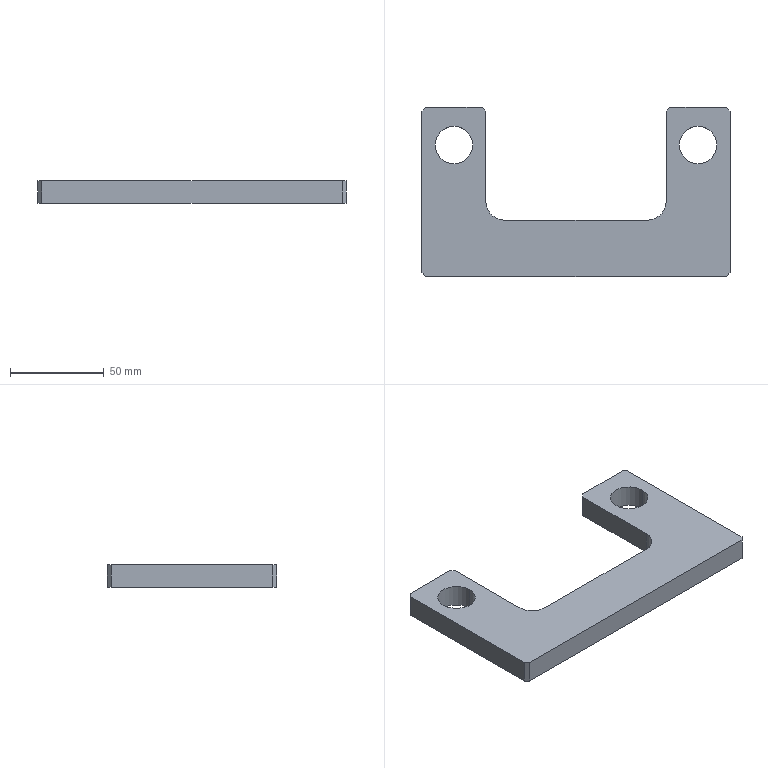Part | SolidWorks | features Chamfer 1, Extrusion 1, Fillet 1 | 1 solid | 22 faces | box 164 x 90 x 12 mm | volume 100831 mm3 | plane 16 | cylinder 6 | commonest cylinder face diameters 20 x6
STEP:
#1=CARTESIAN_POINT('',(55.,0.,6.));
#2=VERTEX_POINT('',#1);
#3=CARTESIAN_POINT('',(75.,0.,6.));
#4=VERTEX_POINT('',#3);
#5=CARTESIAN_POINT('',(65.,0.,6.));
#6=DIRECTION('',(0.,0.,1.));
#7=DIRECTION('',(1.,0.,0.));
#8=AXIS2_PLACEMENT_3D('',#5,#6,#7);
#9=CIRCLE('',#8,10.);
#10=EDGE_CURVE('',#2,#4,#9,.T.);
#11=ORIENTED_EDGE('',*,*,#10,.T.);
#12=CARTESIAN_POINT('',(75.,0.,-6.));
#13=VERTEX_POINT('',#12);
#14=CARTESIAN_POINT('',(75.,0.,6.));
#15=DIRECTION('',(0.,0.,-1.));
#16=VECTOR('',#15,1000.);
#17=LINE('',#14,#16);
#18=EDGE_CURVE('',#4,#13,#17,.T.);
#19=ORIENTED_EDGE('',*,*,#18,.T.);
#20=CARTESIAN_POINT('',(55.,0.,-6.));
#21=VERTEX_POINT('',#20);
#22=CARTESIAN_POINT('',(65.,0.,-6.));
#23=DIRECTION('',(0.,0.,1.));
#24=DIRECTION('',(1.,0.,0.));
#25=AXIS2_PLACEMENT_3D('',#22,#23,#24);
#26=CIRCLE('',#25,10.);
#27=EDGE_CURVE('',#21,#13,#26,.T.);
#28=ORIENTED_EDGE('',*,*,#27,.F.);
#29=CARTESIAN_POINT('',(55.,0.,6.));
#30=DIRECTION('',(0.,0.,-1.));
#31=VECTOR('',#30,1000.);
#32=LINE('',#29,#31);
#33=EDGE_CURVE('',#2,#21,#32,.T.);
#34=ORIENTED_EDGE('',*,*,#33,.F.);
#35=EDGE_LOOP('',(#11,#19,#28,#34));
#36=FACE_OUTER_BOUND('',#35,.T.);
#37=CARTESIAN_POINT('',(65.,0.,6.));
#38=DIRECTION('',(0.,0.,-1.));
#39=DIRECTION('',(-1.,0.,0.));
#40=AXIS2_PLACEMENT_3D('',#37,#38,#39);
#41=CYLINDRICAL_SURFACE('',#40,10.);
#42=ADVANCED_FACE('',(#36),#41,.F.);
#43=CARTESIAN_POINT('',(-75.,0.,6.));
#44=VERTEX_POINT('',#43);
#45=CARTESIAN_POINT('',(-55.,0.,6.));
#46=VERTEX_POINT('',#45);
#47=CARTESIAN_POINT('',(-65.,0.,6.));
#48=DIRECTION('',(0.,0.,1.));
#49=DIRECTION('',(1.,0.,0.));
#50=AXIS2_PLACEMENT_3D('',#47,#48,#49);
#51=CIRCLE('',#50,10.);
#52=EDGE_CURVE('',#44,#46,#51,.T.);
#53=ORIENTED_EDGE('',*,*,#52,.T.);
#54=CARTESIAN_POINT('',(-55.,0.,-6.));
#55=VERTEX_POINT('',#54);
#56=CARTESIAN_POINT('',(-55.,0.,6.));
#57=DIRECTION('',(0.,0.,-1.));
#58=VECTOR('',#57,1000.);
#59=LINE('',#56,#58);
#60=EDGE_CURVE('',#46,#55,#59,.T.);
#61=ORIENTED_EDGE('',*,*,#60,.T.);
#62=CARTESIAN_POINT('',(-75.,0.,-6.));
#63=VERTEX_POINT('',#62);
#64=CARTESIAN_POINT('',(-65.,0.,-6.));
#65=DIRECTION('',(0.,0.,1.));
#66=DIRECTION('',(1.,0.,0.));
#67=AXIS2_PLACEMENT_3D('',#64,#65,#66);
#68=CIRCLE('',#67,10.);
#69=EDGE_CURVE('',#63,#55,#68,.T.);
#70=ORIENTED_EDGE('',*,*,#69,.F.);
#71=CARTESIAN_POINT('',(-75.,0.,6.));
#72=DIRECTION('',(0.,0.,-1.));
#73=VECTOR('',#72,1000.);
#74=LINE('',#71,#73);
#75=EDGE_CURVE('',#44,#63,#74,.T.);
#76=ORIENTED_EDGE('',*,*,#75,.F.);
#77=EDGE_LOOP('',(#53,#61,#70,#76));
#78=FACE_OUTER_BOUND('',#77,.T.);
#79=CARTESIAN_POINT('',(-65.,0.,6.));
#80=DIRECTION('',(0.,0.,-1.));
#81=DIRECTION('',(-1.,0.,0.));
#82=AXIS2_PLACEMENT_3D('',#79,#80,#81);
#83=CYLINDRICAL_SURFACE('',#82,10.);
#84=ADVANCED_FACE('',(#78),#83,.F.);
#85=CARTESIAN_POINT('',(-80.,-70.,6.));
#86=VERTEX_POINT('',#85);
#87=CARTESIAN_POINT('',(80.,-70.,6.));
#88=VERTEX_POINT('',#87);
#89=CARTESIAN_POINT('',(82.,-70.,6.));
#90=DIRECTION('',(1.,0.,0.));
#91=VECTOR('',#90,1000.);
#92=LINE('',#89,#91);
#93=EDGE_CURVE('',#86,#88,#92,.T.);
#94=ORIENTED_EDGE('',*,*,#93,.T.);
#95=CARTESIAN_POINT('',(82.,-68.,6.));
#96=VERTEX_POINT('',#95);
#97=CARTESIAN_POINT('',(82.,-68.,6.));
#98=DIRECTION('',(0.7071,0.7071,0.));
#99=VECTOR('',#98,1000.);
#100=LINE('',#97,#99);
#101=EDGE_CURVE('',#88,#96,#100,.T.);
#102=ORIENTED_EDGE('',*,*,#101,.T.);
#103=CARTESIAN_POINT('',(82.,18.,6.));
#104=VERTEX_POINT('',#103);
#105=CARTESIAN_POINT('',(82.,20.,6.));
#106=DIRECTION('',(0.,1.,0.));
#107=VECTOR('',#106,1000.);
#108=LINE('',#105,#107);
#109=EDGE_CURVE('',#96,#104,#108,.T.);
#110=ORIENTED_EDGE('',*,*,#109,.T.);
#111=CARTESIAN_POINT('',(80.,20.,6.));
#112=VERTEX_POINT('',#111);
#113=CARTESIAN_POINT('',(80.,20.,6.));
#114=DIRECTION('',(-0.7071,0.7071,0.));
#115=VECTOR('',#114,1000.);
#116=LINE('',#113,#115);
#117=EDGE_CURVE('',#104,#112,#116,.T.);
#118=ORIENTED_EDGE('',*,*,#117,.T.);
#119=CARTESIAN_POINT('',(50.,20.,6.));
#120=VERTEX_POINT('',#119);
#121=CARTESIAN_POINT('',(48.,20.,6.));
#122=DIRECTION('',(-1.,0.,0.));
#123=VECTOR('',#122,1000.);
#124=LINE('',#121,#123);
#125=EDGE_CURVE('',#112,#120,#124,.T.);
#126=ORIENTED_EDGE('',*,*,#125,.T.);
#127=CARTESIAN_POINT('',(48.,18.,6.));
#128=VERTEX_POINT('',#127);
#129=CARTESIAN_POINT('',(48.,18.,6.));
#130=DIRECTION('',(-0.7071,-0.7071,0.));
#131=VECTOR('',#130,1000.);
#132=LINE('',#129,#131);
#133=EDGE_CURVE('',#120,#128,#132,.T.);
#134=ORIENTED_EDGE('',*,*,#133,.T.);
#135=CARTESIAN_POINT('',(48.,-30.,6.));
#136=VERTEX_POINT('',#135);
#137=CARTESIAN_POINT('',(48.,-40.,6.));
#138=DIRECTION('',(0.,-1.,0.));
#139=VECTOR('',#138,1000.);
#140=LINE('',#137,#139);
#141=EDGE_CURVE('',#128,#136,#140,.T.);
#142=ORIENTED_EDGE('',*,*,#141,.T.);
#143=CARTESIAN_POINT('',(38.,-40.,6.));
#144=VERTEX_POINT('',#143);
#145=CARTESIAN_POINT('',(38.,-30.,6.));
#146=DIRECTION('',(0.,0.,-1.));
#147=DIRECTION('',(-1.,0.,0.));
#148=AXIS2_PLACEMENT_3D('',#145,#146,#147);
#149=CIRCLE('',#148,10.);
#150=EDGE_CURVE('',#136,#144,#149,.T.);
#151=ORIENTED_EDGE('',*,*,#150,.T.);
#152=CARTESIAN_POINT('',(-38.,-40.,6.));
#153=VERTEX_POINT('',#152);
#154=CARTESIAN_POINT('',(-48.,-40.,6.));
#155=DIRECTION('',(-1.,0.,0.));
#156=VECTOR('',#155,1000.);
#157=LINE('',#154,#156);
#158=EDGE_CURVE('',#144,#153,#157,.T.);
#159=ORIENTED_EDGE('',*,*,#158,.T.);
#160=CARTESIAN_POINT('',(-48.,-30.,6.));
#161=VERTEX_POINT('',#160);
#162=CARTESIAN_POINT('',(-38.,-30.,6.));
#163=DIRECTION('',(0.,0.,-1.));
#164=DIRECTION('',(-1.,0.,0.));
#165=AXIS2_PLACEMENT_3D('',#162,#163,#164);
#166=CIRCLE('',#165,10.);
#167=EDGE_CURVE('',#153,#161,#166,.T.);
#168=ORIENTED_EDGE('',*,*,#167,.T.);
#169=CARTESIAN_POINT('',(-48.,18.,6.));
#170=VERTEX_POINT('',#169);
#171=CARTESIAN_POINT('',(-48.,20.,6.));
#172=DIRECTION('',(0.,1.,0.));
#173=VECTOR('',#172,1000.);
#174=LINE('',#171,#173);
#175=EDGE_CURVE('',#161,#170,#174,.T.);
#176=ORIENTED_EDGE('',*,*,#175,.T.);
#177=CARTESIAN_POINT('',(-50.,20.,6.));
#178=VERTEX_POINT('',#177);
#179=CARTESIAN_POINT('',(-50.,20.,6.));
#180=DIRECTION('',(-0.7071,0.7071,0.));
#181=VECTOR('',#180,1000.);
#182=LINE('',#179,#181);
#183=EDGE_CURVE('',#170,#178,#182,.T.);
#184=ORIENTED_EDGE('',*,*,#183,.T.);
#185=CARTESIAN_POINT('',(-80.,20.,6.));
#186=VERTEX_POINT('',#185);
#187=CARTESIAN_POINT('',(-82.,20.,6.));
#188=DIRECTION('',(-1.,0.,0.));
#189=VECTOR('',#188,1000.);
#190=LINE('',#187,#189);
#191=EDGE_CURVE('',#178,#186,#190,.T.);
#192=ORIENTED_EDGE('',*,*,#191,.T.);
#193=CARTESIAN_POINT('',(-82.,18.,6.));
#194=VERTEX_POINT('',#193);
#195=CARTESIAN_POINT('',(-82.,18.,6.));
#196=DIRECTION('',(-0.7071,-0.7071,0.));
#197=VECTOR('',#196,1000.);
#198=LINE('',#195,#197);
#199=EDGE_CURVE('',#186,#194,#198,.T.);
#200=ORIENTED_EDGE('',*,*,#199,.T.);
#201=CARTESIAN_POINT('',(-82.,-68.,6.));
#202=VERTEX_POINT('',#201);
#203=CARTESIAN_POINT('',(-82.,-70.,6.));
#204=DIRECTION('',(0.,-1.,0.));
#205=VECTOR('',#204,1000.);
#206=LINE('',#203,#205);
#207=EDGE_CURVE('',#194,#202,#206,.T.);
#208=ORIENTED_EDGE('',*,*,#207,.T.);
#209=CARTESIAN_POINT('',(-80.,-70.,6.));
#210=DIRECTION('',(0.7071,-0.7071,0.));
#211=VECTOR('',#210,1000.);
#212=LINE('',#209,#211);
#213=EDGE_CURVE('',#202,#86,#212,.T.);
#214=ORIENTED_EDGE('',*,*,#213,.T.);
#215=EDGE_LOOP('',(#94,#102,#110,#118,#126,#134,#142,#151,#159,#168,#176,#184,#192,#200,#208,#214));
#216=FACE_OUTER_BOUND('',#215,.T.);
#217=ORIENTED_EDGE('',*,*,#52,.F.);
#218=CARTESIAN_POINT('',(-65.,0.,6.));
#219=DIRECTION('',(0.,0.,1.));
#220=DIRECTION('',(1.,0.,0.));
#221=AXIS2_PLACEMENT_3D('',#218,#219,#220);
#222=CIRCLE('',#221,10.);
#223=EDGE_CURVE('',#46,#44,#222,.T.);
#224=ORIENTED_EDGE('',*,*,#223,.F.);
#225=EDGE_LOOP('',(#217,#224));
#226=FACE_BOUND('',#225,.T.);
#227=ORIENTED_EDGE('',*,*,#10,.F.);
#228=CARTESIAN_POINT('',(65.,0.,6.));
#229=DIRECTION('',(0.,0.,1.));
#230=DIRECTION('',(1.,0.,0.));
#231=AXIS2_PLACEMENT_3D('',#228,#229,#230);
#232=CIRCLE('',#231,10.);
#233=EDGE_CURVE('',#4,#2,#232,.T.);
#234=ORIENTED_EDGE('',*,*,#233,.F.);
#235=EDGE_LOOP('',(#227,#234));
#236=FACE_BOUND('',#235,.T.);
#237=CARTESIAN_POINT('',(0.,0.,6.));
#238=DIRECTION('',(0.,0.,-1.));
#239=DIRECTION('',(-1.,0.,0.));
#240=AXIS2_PLACEMENT_3D('',#237,#238,#239);
#241=PLANE('',#240);
#242=ADVANCED_FACE('',(#216,#226,#236),#241,.F.);
#243=ORIENTED_EDGE('',*,*,#69,.T.);
#244=CARTESIAN_POINT('',(-65.,0.,-6.));
#245=DIRECTION('',(0.,0.,1.));
#246=DIRECTION('',(1.,0.,0.));
#247=AXIS2_PLACEMENT_3D('',#244,#245,#246);
#248=CIRCLE('',#247,10.);
#249=EDGE_CURVE('',#55,#63,#248,.T.);
#250=ORIENTED_EDGE('',*,*,#249,.T.);
#251=EDGE_LOOP('',(#243,#250));
#252=FACE_BOUND('',#251,.T.);
#253=CARTESIAN_POINT('',(82.,-68.,-6.));
#254=VERTEX_POINT('',#253);
#255=CARTESIAN_POINT('',(82.,18.,-6.));
#256=VERTEX_POINT('',#255);
#257=CARTESIAN_POINT('',(82.,20.,-6.));
#258=DIRECTION('',(0.,1.,0.));
#259=VECTOR('',#258,1000.);
#260=LINE('',#257,#259);
#261=EDGE_CURVE('',#254,#256,#260,.T.);
#262=ORIENTED_EDGE('',*,*,#261,.F.);
#263=CARTESIAN_POINT('',(80.,-70.,-6.));
#264=VERTEX_POINT('',#263);
#265=CARTESIAN_POINT('',(75.,-75.,-6.));
#266=DIRECTION('',(-0.7071,-0.7071,0.));
#267=VECTOR('',#266,1000.);
#268=LINE('',#265,#267);
#269=EDGE_CURVE('',#254,#264,#268,.T.);
#270=ORIENTED_EDGE('',*,*,#269,.T.);
#271=CARTESIAN_POINT('',(-80.,-70.,-6.));
#272=VERTEX_POINT('',#271);
#273=CARTESIAN_POINT('',(82.,-70.,-6.));
#274=DIRECTION('',(1.,0.,0.));
#275=VECTOR('',#274,1000.);
#276=LINE('',#273,#275);
#277=EDGE_CURVE('',#272,#264,#276,.T.);
#278=ORIENTED_EDGE('',*,*,#277,.F.);
#279=CARTESIAN_POINT('',(-82.,-68.,-6.));
#280=VERTEX_POINT('',#279);
#281=CARTESIAN_POINT('',(-75.,-75.,-6.));
#282=DIRECTION('',(-0.7071,0.7071,0.));
#283=VECTOR('',#282,1000.);
#284=LINE('',#281,#283);
#285=EDGE_CURVE('',#272,#280,#284,.T.);
#286=ORIENTED_EDGE('',*,*,#285,.T.);
#287=CARTESIAN_POINT('',(-82.,18.,-6.));
#288=VERTEX_POINT('',#287);
#289=CARTESIAN_POINT('',(-82.,-70.,-6.));
#290=DIRECTION('',(0.,-1.,0.));
#291=VECTOR('',#290,1000.);
#292=LINE('',#289,#291);
#293=EDGE_CURVE('',#288,#280,#292,.T.);
#294=ORIENTED_EDGE('',*,*,#293,.F.);
#295=CARTESIAN_POINT('',(-80.,20.,-6.));
#296=VERTEX_POINT('',#295);
#297=CARTESIAN_POINT('',(-50.,50.,-6.));
#298=DIRECTION('',(0.7071,0.7071,0.));
#299=VECTOR('',#298,1000.);
#300=LINE('',#297,#299);
#301=EDGE_CURVE('',#288,#296,#300,.T.);
#302=ORIENTED_EDGE('',*,*,#301,.T.);
#303=CARTESIAN_POINT('',(-50.,20.,-6.));
#304=VERTEX_POINT('',#303);
#305=CARTESIAN_POINT('',(-82.,20.,-6.));
#306=DIRECTION('',(-1.,0.,0.));
#307=VECTOR('',#306,1000.);
#308=LINE('',#305,#307);
#309=EDGE_CURVE('',#304,#296,#308,.T.);
#310=ORIENTED_EDGE('',*,*,#309,.F.);
#311=CARTESIAN_POINT('',(-48.,18.,-6.));
#312=VERTEX_POINT('',#311);
#313=CARTESIAN_POINT('',(-15.,-15.,-6.));
#314=DIRECTION('',(0.7071,-0.7071,0.));
#315=VECTOR('',#314,1000.);
#316=LINE('',#313,#315);
#317=EDGE_CURVE('',#304,#312,#316,.T.);
#318=ORIENTED_EDGE('',*,*,#317,.T.);
#319=CARTESIAN_POINT('',(-48.,-30.,-6.));
#320=VERTEX_POINT('',#319);
#321=CARTESIAN_POINT('',(-48.,20.,-6.));
#322=DIRECTION('',(0.,1.,0.));
#323=VECTOR('',#322,1000.);
#324=LINE('',#321,#323);
#325=EDGE_CURVE('',#320,#312,#324,.T.);
#326=ORIENTED_EDGE('',*,*,#325,.F.);
#327=CARTESIAN_POINT('',(-38.,-40.,-6.));
#328=VERTEX_POINT('',#327);
#329=CARTESIAN_POINT('',(-38.,-30.,-6.));
#330=DIRECTION('',(0.,0.,1.));
#331=DIRECTION('',(-1.,0.,0.));
#332=AXIS2_PLACEMENT_3D('',#329,#330,#331);
#333=CIRCLE('',#332,10.);
#334=EDGE_CURVE('',#320,#328,#333,.T.);
#335=ORIENTED_EDGE('',*,*,#334,.T.);
#336=CARTESIAN_POINT('',(38.,-40.,-6.));
#337=VERTEX_POINT('',#336);
#338=CARTESIAN_POINT('',(-48.,-40.,-6.));
#339=DIRECTION('',(-1.,0.,0.));
#340=VECTOR('',#339,1000.);
#341=LINE('',#338,#340);
#342=EDGE_CURVE('',#337,#328,#341,.T.);
#343=ORIENTED_EDGE('',*,*,#342,.F.);
#344=CARTESIAN_POINT('',(48.,-30.,-6.));
#345=VERTEX_POINT('',#344);
#346=CARTESIAN_POINT('',(38.,-30.,-6.));
#347=DIRECTION('',(0.,0.,1.));
#348=DIRECTION('',(-1.,0.,0.));
#349=AXIS2_PLACEMENT_3D('',#346,#347,#348);
#350=CIRCLE('',#349,10.);
#351=EDGE_CURVE('',#337,#345,#350,.T.);
#352=ORIENTED_EDGE('',*,*,#351,.T.);
#353=CARTESIAN_POINT('',(48.,18.,-6.));
#354=VERTEX_POINT('',#353);
#355=CARTESIAN_POINT('',(48.,-40.,-6.));
#356=DIRECTION('',(0.,-1.,0.));
#357=VECTOR('',#356,1000.);
#358=LINE('',#355,#357);
#359=EDGE_CURVE('',#354,#345,#358,.T.);
#360=ORIENTED_EDGE('',*,*,#359,.F.);
#361=CARTESIAN_POINT('',(50.,20.,-6.));
#362=VERTEX_POINT('',#361);
#363=CARTESIAN_POINT('',(15.,-15.,-6.));
#364=DIRECTION('',(0.7071,0.7071,0.));
#365=VECTOR('',#364,1000.);
#366=LINE('',#363,#365);
#367=EDGE_CURVE('',#354,#362,#366,.T.);
#368=ORIENTED_EDGE('',*,*,#367,.T.);
#369=CARTESIAN_POINT('',(80.,20.,-6.));
#370=VERTEX_POINT('',#369);
#371=CARTESIAN_POINT('',(48.,20.,-6.));
#372=DIRECTION('',(-1.,0.,0.));
#373=VECTOR('',#372,1000.);
#374=LINE('',#371,#373);
#375=EDGE_CURVE('',#370,#362,#374,.T.);
#376=ORIENTED_EDGE('',*,*,#375,.F.);
#377=CARTESIAN_POINT('',(50.,50.,-6.));
#378=DIRECTION('',(0.7071,-0.7071,0.));
#379=VECTOR('',#378,1000.);
#380=LINE('',#377,#379);
#381=EDGE_CURVE('',#370,#256,#380,.T.);
#382=ORIENTED_EDGE('',*,*,#381,.T.);
#383=EDGE_LOOP('',(#262,#270,#278,#286,#294,#302,#310,#318,#326,#335,#343,#352,#360,#368,#376,#382));
#384=FACE_OUTER_BOUND('',#383,.T.);
#385=ORIENTED_EDGE('',*,*,#27,.T.);
#386=CARTESIAN_POINT('',(65.,0.,-6.));
#387=DIRECTION('',(0.,0.,1.));
#388=DIRECTION('',(1.,0.,0.));
#389=AXIS2_PLACEMENT_3D('',#386,#387,#388);
#390=CIRCLE('',#389,10.);
#391=EDGE_CURVE('',#13,#21,#390,.T.);
#392=ORIENTED_EDGE('',*,*,#391,.T.);
#393=EDGE_LOOP('',(#385,#392));
#394=FACE_BOUND('',#393,.T.);
#395=CARTESIAN_POINT('',(0.,0.,-6.));
#396=DIRECTION('',(0.,0.,-1.));
#397=DIRECTION('',(-1.,0.,0.));
#398=AXIS2_PLACEMENT_3D('',#395,#396,#397);
#399=PLANE('',#398);
#400=ADVANCED_FACE('',(#252,#384,#394),#399,.T.);
#401=ORIENTED_EDGE('',*,*,#191,.F.);
#402=CARTESIAN_POINT('',(-50.,20.,6.));
#403=DIRECTION('',(0.,0.,-1.));
#404=VECTOR('',#403,1000.);
#405=LINE('',#402,#404);
#406=EDGE_CURVE('',#178,#304,#405,.T.);
#407=ORIENTED_EDGE('',*,*,#406,.T.);
#408=ORIENTED_EDGE('',*,*,#309,.T.);
#409=CARTESIAN_POINT('',(-80.,20.,6.));
#410=DIRECTION('',(0.,0.,1.));
#411=VECTOR('',#410,1000.);
#412=LINE('',#409,#411);
#413=EDGE_CURVE('',#296,#186,#412,.T.);
#414=ORIENTED_EDGE('',*,*,#413,.T.);
#415=EDGE_LOOP('',(#401,#407,#408,#414));
#416=FACE_OUTER_BOUND('',#415,.T.);
#417=CARTESIAN_POINT('',(-82.,20.,6.));
#418=DIRECTION('',(0.,-1.,0.));
#419=DIRECTION('',(0.,0.,-1.));
#420=AXIS2_PLACEMENT_3D('',#417,#418,#419);
#421=PLANE('',#420);
#422=ADVANCED_FACE('',(#416),#421,.F.);
#423=ORIENTED_EDGE('',*,*,#293,.T.);
#424=CARTESIAN_POINT('',(-82.,-68.,6.));
#425=DIRECTION('',(0.,0.,1.));
#426=VECTOR('',#425,1000.);
#427=LINE('',#424,#426);
#428=EDGE_CURVE('',#280,#202,#427,.T.);
#429=ORIENTED_EDGE('',*,*,#428,.T.);
#430=ORIENTED_EDGE('',*,*,#207,.F.);
#431=CARTESIAN_POINT('',(-82.,18.,6.));
#432=DIRECTION('',(0.,0.,-1.));
#433=VECTOR('',#432,1000.);
#434=LINE('',#431,#433);
#435=EDGE_CURVE('',#194,#288,#434,.T.);
#436=ORIENTED_EDGE('',*,*,#435,.T.);
#437=EDGE_LOOP('',(#423,#429,#430,#436));
#438=FACE_OUTER_BOUND('',#437,.T.);
#439=CARTESIAN_POINT('',(-82.,-70.,6.));
#440=DIRECTION('',(1.,0.,0.));
#441=DIRECTION('',(0.,1.,0.));
#442=AXIS2_PLACEMENT_3D('',#439,#440,#441);
#443=PLANE('',#442);
#444=ADVANCED_FACE('',(#438),#443,.F.);
#445=ORIENTED_EDGE('',*,*,#277,.T.);
#446=CARTESIAN_POINT('',(80.,-70.,6.));
#447=DIRECTION('',(0.,0.,1.));
#448=VECTOR('',#447,1000.);
#449=LINE('',#446,#448);
#450=EDGE_CURVE('',#264,#88,#449,.T.);
#451=ORIENTED_EDGE('',*,*,#450,.T.);
#452=ORIENTED_EDGE('',*,*,#93,.F.);
#453=CARTESIAN_POINT('',(-80.,-70.,6.));
#454=DIRECTION('',(0.,0.,-1.));
#455=VECTOR('',#454,1000.);
#456=LINE('',#453,#455);
#457=EDGE_CURVE('',#86,#272,#456,.T.);
#458=ORIENTED_EDGE('',*,*,#457,.T.);
#459=EDGE_LOOP('',(#445,#451,#452,#458));
#460=FACE_OUTER_BOUND('',#459,.T.);
#461=CARTESIAN_POINT('',(82.,-70.,6.));
#462=DIRECTION('',(0.,1.,0.));
#463=DIRECTION('',(-1.,0.,0.));
#464=AXIS2_PLACEMENT_3D('',#461,#462,#463);
#465=PLANE('',#464);
#466=ADVANCED_FACE('',(#460),#465,.F.);
#467=ORIENTED_EDGE('',*,*,#109,.F.);
#468=CARTESIAN_POINT('',(82.,-68.,6.));
#469=DIRECTION('',(0.,0.,-1.));
#470=VECTOR('',#469,1000.);
#471=LINE('',#468,#470);
#472=EDGE_CURVE('',#96,#254,#471,.T.);
#473=ORIENTED_EDGE('',*,*,#472,.T.);
#474=ORIENTED_EDGE('',*,*,#261,.T.);
#475=CARTESIAN_POINT('',(82.,18.,6.));
#476=DIRECTION('',(0.,0.,1.));
#477=VECTOR('',#476,1000.);
#478=LINE('',#475,#477);
#479=EDGE_CURVE('',#256,#104,#478,.T.);
#480=ORIENTED_EDGE('',*,*,#479,.T.);
#481=EDGE_LOOP('',(#467,#473,#474,#480));
#482=FACE_OUTER_BOUND('',#481,.T.);
#483=CARTESIAN_POINT('',(82.,20.,6.));
#484=DIRECTION('',(-1.,0.,0.));
#485=DIRECTION('',(0.,-1.,0.));
#486=AXIS2_PLACEMENT_3D('',#483,#484,#485);
#487=PLANE('',#486);
#488=ADVANCED_FACE('',(#482),#487,.F.);
#489=ORIENTED_EDGE('',*,*,#125,.F.);
#490=CARTESIAN_POINT('',(80.,20.,6.));
#491=DIRECTION('',(0.,0.,-1.));
#492=VECTOR('',#491,1000.);
#493=LINE('',#490,#492);
#494=EDGE_CURVE('',#112,#370,#493,.T.);
#495=ORIENTED_EDGE('',*,*,#494,.T.);
#496=ORIENTED_EDGE('',*,*,#375,.T.);
#497=CARTESIAN_POINT('',(50.,20.,6.));
#498=DIRECTION('',(0.,0.,1.));
#499=VECTOR('',#498,1000.);
#500=LINE('',#497,#499);
#501=EDGE_CURVE('',#362,#120,#500,.T.);
#502=ORIENTED_EDGE('',*,*,#501,.T.);
#503=EDGE_LOOP('',(#489,#495,#496,#502));
#504=FACE_OUTER_BOUND('',#503,.T.);
#505=CARTESIAN_POINT('',(48.,20.,6.));
#506=DIRECTION('',(0.,-1.,0.));
#507=DIRECTION('',(0.,0.,-1.));
#508=AXIS2_PLACEMENT_3D('',#505,#506,#507);
#509=PLANE('',#508);
#510=ADVANCED_FACE('',(#504),#509,.F.);
#511=ORIENTED_EDGE('',*,*,#141,.F.);
#512=CARTESIAN_POINT('',(48.,18.,6.));
#513=DIRECTION('',(0.,0.,-1.));
#514=VECTOR('',#513,1000.);
#515=LINE('',#512,#514);
#516=EDGE_CURVE('',#128,#354,#515,.T.);
#517=ORIENTED_EDGE('',*,*,#516,.T.);
#518=ORIENTED_EDGE('',*,*,#359,.T.);
#519=CARTESIAN_POINT('',(48.,-30.,6.));
#520=DIRECTION('',(0.,0.,1.));
#521=VECTOR('',#520,1000.);
#522=LINE('',#519,#521);
#523=EDGE_CURVE('',#345,#136,#522,.T.);
#524=ORIENTED_EDGE('',*,*,#523,.T.);
#525=EDGE_LOOP('',(#511,#517,#518,#524));
#526=FACE_OUTER_BOUND('',#525,.T.);
#527=CARTESIAN_POINT('',(48.,-40.,6.));
#528=DIRECTION('',(1.,0.,0.));
#529=DIRECTION('',(0.,1.,0.));
#530=AXIS2_PLACEMENT_3D('',#527,#528,#529);
#531=PLANE('',#530);
#532=ADVANCED_FACE('',(#526),#531,.F.);
#533=ORIENTED_EDGE('',*,*,#158,.F.);
#534=CARTESIAN_POINT('',(38.,-40.,-6.));
#535=DIRECTION('',(0.,0.,-1.));
#536=VECTOR('',#535,1000.);
#537=LINE('',#534,#536);
#538=EDGE_CURVE('',#144,#337,#537,.T.);
#539=ORIENTED_EDGE('',*,*,#538,.T.);
#540=ORIENTED_EDGE('',*,*,#342,.T.);
#541=CARTESIAN_POINT('',(-38.,-40.,6.));
#542=DIRECTION('',(0.,0.,1.));
#543=VECTOR('',#542,1000.);
#544=LINE('',#541,#543);
#545=EDGE_CURVE('',#328,#153,#544,.T.);
#546=ORIENTED_EDGE('',*,*,#545,.T.);
#547=EDGE_LOOP('',(#533,#539,#540,#546));
#548=FACE_OUTER_BOUND('',#547,.T.);
#549=CARTESIAN_POINT('',(-48.,-40.,6.));
#550=DIRECTION('',(0.,-1.,0.));
#551=DIRECTION('',(0.,0.,-1.));
#552=AXIS2_PLACEMENT_3D('',#549,#550,#551);
#553=PLANE('',#552);
#554=ADVANCED_FACE('',(#548),#553,.F.);
#555=ORIENTED_EDGE('',*,*,#325,.T.);
#556=CARTESIAN_POINT('',(-48.,18.,6.));
#557=DIRECTION('',(0.,0.,1.));
#558=VECTOR('',#557,1000.);
#559=LINE('',#556,#558);
#560=EDGE_CURVE('',#312,#170,#559,.T.);
#561=ORIENTED_EDGE('',*,*,#560,.T.);
#562=ORIENTED_EDGE('',*,*,#175,.F.);
#563=CARTESIAN_POINT('',(-48.,-30.,-6.));
#564=DIRECTION('',(0.,0.,-1.));
#565=VECTOR('',#564,1000.);
#566=LINE('',#563,#565);
#567=EDGE_CURVE('',#161,#320,#566,.T.);
#568=ORIENTED_EDGE('',*,*,#567,.T.);
#569=EDGE_LOOP('',(#555,#561,#562,#568));
#570=FACE_OUTER_BOUND('',#569,.T.);
#571=CARTESIAN_POINT('',(-48.,20.,6.));
#572=DIRECTION('',(-1.,0.,0.));
#573=DIRECTION('',(0.,-1.,0.));
#574=AXIS2_PLACEMENT_3D('',#571,#572,#573);
#575=PLANE('',#574);
#576=ADVANCED_FACE('',(#570),#575,.F.);
#577=ORIENTED_EDGE('',*,*,#60,.F.);
#578=ORIENTED_EDGE('',*,*,#223,.T.);
#579=ORIENTED_EDGE('',*,*,#75,.T.);
#580=ORIENTED_EDGE('',*,*,#249,.F.);
#581=EDGE_LOOP('',(#577,#578,#579,#580));
#582=FACE_OUTER_BOUND('',#581,.T.);
#583=CARTESIAN_POINT('',(-65.,0.,6.));
#584=DIRECTION('',(0.,0.,-1.));
#585=DIRECTION('',(-1.,0.,0.));
#586=AXIS2_PLACEMENT_3D('',#583,#584,#585);
#587=CYLINDRICAL_SURFACE('',#586,10.);
#588=ADVANCED_FACE('',(#582),#587,.F.);
#589=ORIENTED_EDGE('',*,*,#18,.F.);
#590=ORIENTED_EDGE('',*,*,#233,.T.);
#591=ORIENTED_EDGE('',*,*,#33,.T.);
#592=ORIENTED_EDGE('',*,*,#391,.F.);
#593=EDGE_LOOP('',(#589,#590,#591,#592));
#594=FACE_OUTER_BOUND('',#593,.T.);
#595=CARTESIAN_POINT('',(65.,0.,6.));
#596=DIRECTION('',(0.,0.,-1.));
#597=DIRECTION('',(-1.,0.,0.));
#598=AXIS2_PLACEMENT_3D('',#595,#596,#597);
#599=CYLINDRICAL_SURFACE('',#598,10.);
#600=ADVANCED_FACE('',(#594),#599,.F.);
#601=ORIENTED_EDGE('',*,*,#150,.F.);
#602=ORIENTED_EDGE('',*,*,#523,.F.);
#603=ORIENTED_EDGE('',*,*,#351,.F.);
#604=ORIENTED_EDGE('',*,*,#538,.F.);
#605=EDGE_LOOP('',(#601,#602,#603,#604));
#606=FACE_OUTER_BOUND('',#605,.T.);
#607=CARTESIAN_POINT('',(38.,-30.,6.));
#608=DIRECTION('',(0.,0.,1.));
#609=DIRECTION('',(1.,0.,0.));
#610=AXIS2_PLACEMENT_3D('',#607,#608,#609);
#611=CYLINDRICAL_SURFACE('',#610,10.);
#612=ADVANCED_FACE('',(#606),#611,.F.);
#613=ORIENTED_EDGE('',*,*,#167,.F.);
#614=ORIENTED_EDGE('',*,*,#545,.F.);
#615=ORIENTED_EDGE('',*,*,#334,.F.);
#616=ORIENTED_EDGE('',*,*,#567,.F.);
#617=EDGE_LOOP('',(#613,#614,#615,#616));
#618=FACE_OUTER_BOUND('',#617,.T.);
#619=CARTESIAN_POINT('',(-38.,-30.,6.));
#620=DIRECTION('',(0.,0.,1.));
#621=DIRECTION('',(1.,0.,0.));
#622=AXIS2_PLACEMENT_3D('',#619,#620,#621);
#623=CYLINDRICAL_SURFACE('',#622,10.);
#624=ADVANCED_FACE('',(#618),#623,.F.);
#625=ORIENTED_EDGE('',*,*,#101,.F.);
#626=ORIENTED_EDGE('',*,*,#450,.F.);
#627=ORIENTED_EDGE('',*,*,#269,.F.);
#628=ORIENTED_EDGE('',*,*,#472,.F.);
#629=EDGE_LOOP('',(#625,#626,#627,#628));
#630=FACE_OUTER_BOUND('',#629,.T.);
#631=CARTESIAN_POINT('',(82.,-68.,6.));
#632=DIRECTION('',(-0.7071,0.7071,0.));
#633=DIRECTION('',(0.,0.,-1.));
#634=AXIS2_PLACEMENT_3D('',#631,#632,#633);
#635=PLANE('',#634);
#636=ADVANCED_FACE('',(#630),#635,.F.);
#637=ORIENTED_EDGE('',*,*,#213,.F.);
#638=ORIENTED_EDGE('',*,*,#428,.F.);
#639=ORIENTED_EDGE('',*,*,#285,.F.);
#640=ORIENTED_EDGE('',*,*,#457,.F.);
#641=EDGE_LOOP('',(#637,#638,#639,#640));
#642=FACE_OUTER_BOUND('',#641,.T.);
#643=CARTESIAN_POINT('',(-80.,-70.,6.));
#644=DIRECTION('',(0.7071,0.7071,0.));
#645=DIRECTION('',(0.,0.,-1.));
#646=AXIS2_PLACEMENT_3D('',#643,#644,#645);
#647=PLANE('',#646);
#648=ADVANCED_FACE('',(#642),#647,.F.);
#649=ORIENTED_EDGE('',*,*,#117,.F.);
#650=ORIENTED_EDGE('',*,*,#479,.F.);
#651=ORIENTED_EDGE('',*,*,#381,.F.);
#652=ORIENTED_EDGE('',*,*,#494,.F.);
#653=EDGE_LOOP('',(#649,#650,#651,#652));
#654=FACE_OUTER_BOUND('',#653,.T.);
#655=CARTESIAN_POINT('',(80.,20.,6.));
#656=DIRECTION('',(-0.7071,-0.7071,0.));
#657=DIRECTION('',(0.,0.,-1.));
#658=AXIS2_PLACEMENT_3D('',#655,#656,#657);
#659=PLANE('',#658);
#660=ADVANCED_FACE('',(#654),#659,.F.);
#661=ORIENTED_EDGE('',*,*,#133,.F.);
#662=ORIENTED_EDGE('',*,*,#501,.F.);
#663=ORIENTED_EDGE('',*,*,#367,.F.);
#664=ORIENTED_EDGE('',*,*,#516,.F.);
#665=EDGE_LOOP('',(#661,#662,#663,#664));
#666=FACE_OUTER_BOUND('',#665,.T.);
#667=CARTESIAN_POINT('',(48.,18.,6.));
#668=DIRECTION('',(0.7071,-0.7071,0.));
#669=DIRECTION('',(0.,0.,-1.));
#670=AXIS2_PLACEMENT_3D('',#667,#668,#669);
#671=PLANE('',#670);
#672=ADVANCED_FACE('',(#666),#671,.F.);
#673=ORIENTED_EDGE('',*,*,#183,.F.);
#674=ORIENTED_EDGE('',*,*,#560,.F.);
#675=ORIENTED_EDGE('',*,*,#317,.F.);
#676=ORIENTED_EDGE('',*,*,#406,.F.);
#677=EDGE_LOOP('',(#673,#674,#675,#676));
#678=FACE_OUTER_BOUND('',#677,.T.);
#679=CARTESIAN_POINT('',(-50.,20.,6.));
#680=DIRECTION('',(-0.7071,-0.7071,0.));
#681=DIRECTION('',(0.,0.,-1.));
#682=AXIS2_PLACEMENT_3D('',#679,#680,#681);
#683=PLANE('',#682);
#684=ADVANCED_FACE('',(#678),#683,.F.);
#685=ORIENTED_EDGE('',*,*,#199,.F.);
#686=ORIENTED_EDGE('',*,*,#413,.F.);
#687=ORIENTED_EDGE('',*,*,#301,.F.);
#688=ORIENTED_EDGE('',*,*,#435,.F.);
#689=EDGE_LOOP('',(#685,#686,#687,#688));
#690=FACE_OUTER_BOUND('',#689,.T.);
#691=CARTESIAN_POINT('',(-82.,18.,6.));
#692=DIRECTION('',(0.7071,-0.7071,0.));
#693=DIRECTION('',(0.,0.,-1.));
#694=AXIS2_PLACEMENT_3D('',#691,#692,#693);
#695=PLANE('',#694);
#696=ADVANCED_FACE('',(#690),#695,.F.);
#697=CLOSED_SHELL('',(#42,#84,#242,#400,#422,#444,#466,#488,#510,#532,#554,#576,#588,#600,#612,#624,#636,#648,#660,#672,#684,#696));
#698=MANIFOLD_SOLID_BREP('',#697);
#699=CARTESIAN_POINT('',(0.,0.,0.));
#700=DIRECTION('',(0.,0.,1.));
#701=DIRECTION('',(1.,0.,0.));
#702=AXIS2_PLACEMENT_3D('',#699,#700,#701);
#703=(LENGTH_UNIT()NAMED_UNIT(*)SI_UNIT(.MILLI.,.METRE.));
#704=UNCERTAINTY_MEASURE_WITH_UNIT(LENGTH_MEASURE(0.00001),#703,'','');
#705=(NAMED_UNIT(*)PLANE_ANGLE_UNIT()SI_UNIT($,.RADIAN.));
#706=(NAMED_UNIT(*)SI_UNIT($,.STERADIAN.)SOLID_ANGLE_UNIT());
#707=(GEOMETRIC_REPRESENTATION_CONTEXT(3)GLOBAL_UNCERTAINTY_ASSIGNED_CONTEXT((#704))GLOBAL_UNIT_ASSIGNED_CONTEXT((#703,#705,#706))REPRESENTATION_CONTEXT('',''));
#708=ADVANCED_BREP_SHAPE_REPRESENTATION('',(#698,#702),#707);